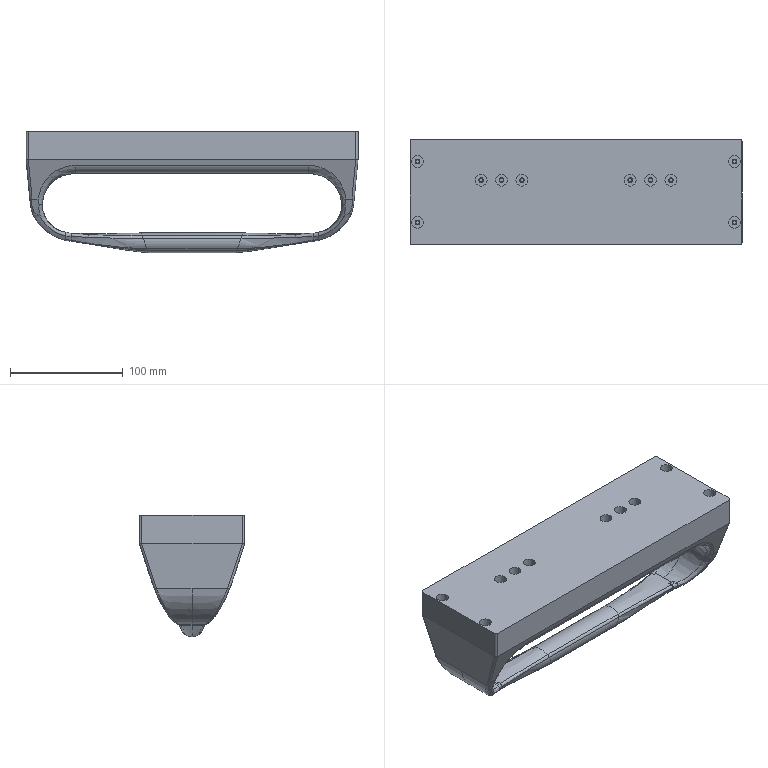NC program | NX | posted with a generic post | part box 294.078 x 93.5 x 107.5 mm
Lines 1 to 258 of 185821:
N10 G17 G21 G94 G90
(ZLEVEL_PROFILE_COPY_COPY_1_COPY_COPY_COPY_COPY_1_COPY , TOOL : D10JING)
N12 T11 M6
N14 G54
N16 G17 G0 G90 X153.539 Y4.496 B0. C0. S7500 M3
N18 G43 Z30. H11
N20 Z-14.083
N22 G94 G1 Z-17.083 F1000.
N24 X153.117 Y4.303
N26 G3 X152.538 Y3.489 R1.
N28 G1 X152.016 Y-1.977
N30 X148.185 Y-41.977
N32 G2 X145.294 Y-52.36 R34.792
N34 X139.783 Y-61.284 R41.542
N36 X129.039 Y-71.069 R47.845
N38 X116.114 Y-77.165 R48.023
N40 X110.357 Y-78.443 R40.705
N42 G1 X107.918 Y-78.805
N44 G3 X84.406 Y-82.6 R3104.615
N46 G2 X61.778 Y-86.214 R2299.005
N48 X52.738 Y-87.55 R870.562
N50 X43.319 Y-88.706 R268.865
N52 X39.042 Y-89. R58.95
N54 G1 X-38.958
N56 G2 X-43.766 Y-88.652 R65.215
N58 X-54.69 Y-87.261 R282.526
N60 X-74.282 Y-84.231 R1365.267
N62 G1 X-80.833 Y-83.169
N64 X-95.124 Y-80.83
N66 X-96.91 Y-80.54
N68 X-107.866 Y-78.799
N70 X-110.27 Y-78.443
N72 G2 X-117.454 Y-76.717 R41.647
N74 X-138.247 Y-63.051 R48.785
N76 X-144.415 Y-54.142 R42.977
N78 X-147.826 Y-44.342 R36.064
N80 X-148.185 Y-41.977 R29.91
N82 G1 X-152.016 Y-1.977
N84 G2 X-152.036 Y-1.675 R5.
N86 G1 X-152.044 Y-1.662
N88 X-152.053 Y-1.578
N90 X-152.539 Y3.496
N92 G3 X-153.119 Y4.31 R1.
N94 G1 X-153.539 Y4.502
N96 Z-14.083
N98 G0 Z30.
N100 X153.539 Y4.495
N102 Z-29.417
N104 G1 Z-32.417
N106 X153.118 Y4.303
N108 G3 X152.538 Y3.489 R1.
N110 G1 X152.016 Y-1.977
N112 X148.185 Y-41.977
N114 G2 X145.589 Y-51.689 R34.666
N116 X140.148 Y-60.823 R41.108
N118 X129.958 Y-70.441 R47.496
N120 X116.114 Y-77.167 R48.183
N122 X110.357 Y-78.443 R40.559
N124 G1 X107.918 Y-78.805
N126 G3 X84.406 Y-82.601 R3047.623
N128 G2 X61.779 Y-86.214 R2288.49
N130 X52.698 Y-87.554 R792.66
N132 X43.319 Y-88.706 R259.673
N134 X39.042 Y-89. R58.502
N136 G1 X-38.958
N138 G2 X-43.766 Y-88.652 R64.859
N140 X-55.824 Y-87.095 R292.145
N142 X-79.047 Y-83.46 R1588.068
N144 G1 X-96.91 Y-80.54
N146 X-107.866 Y-78.799
N148 X-110.27 Y-78.443
N150 G2 X-116.561 Y-77.005 R40.87
N152 X-128.978 Y-71.069 R48.151
N154 X-139.783 Y-61.238 R47.856
N156 X-145.473 Y-51.914 R41.36
N158 X-148.185 Y-41.977 R34.707
N160 G1 X-152.016 Y-1.977
N162 G2 X-152.036 Y-1.675 R5.
N164 G1 X-152.045 Y-1.662
N166 X-152.539 Y3.495
N168 G3 X-153.12 Y4.31 R1.
N170 G1 X-153.54 Y4.501
N172 Z-29.417
N174 G0 Z30.
N176 X153.54 Y4.495
N178 Z-44.75
N180 G1 Z-47.75
N182 X153.119 Y4.303
N184 G3 X152.538 Y3.489 R1.
N186 G1 X152.016 Y-1.977
N188 X148.185 Y-41.977
N190 G2 X145.589 Y-51.69 R34.638
N192 X139.783 Y-61.284 R41.349
N194 X129.512 Y-70.751 R47.668
N196 X117.007 Y-76.892 R48.224
N198 X110.35 Y-78.444 R40.993
N200 G1 X107.918 Y-78.805
N202 G3 X84.406 Y-82.601 R3090.503
N204 G2 X61.779 Y-86.214 R2278.07
N206 X52.698 Y-87.555 R789.646
N208 X43.319 Y-88.707 R261.333
N210 X39.042 Y-89. R58.377
N212 G1 X-38.958
N214 G2 X-43.325 Y-88.698 R61.364
N216 G1 X-44.659 Y-88.557
N218 G2 X-55.824 Y-87.096 R299.771
N220 G1 X-57.164 Y-86.897
N222 G2 X-80.833 Y-83.17 R1733.297
N224 G1 X-96.91 Y-80.541
N226 X-107.866 Y-78.799
N228 X-110.266 Y-78.444
N230 G2 X-115.667 Y-77.272 R39.927
N232 X-128.979 Y-71.069 R48.025
N234 X-139.783 Y-61.238 R47.852
N236 X-145.474 Y-51.914 R41.354
N238 X-148.185 Y-41.977 R34.724
N240 G1 X-152.016 Y-1.977
N242 G2 X-152.036 Y-1.675 R5.
N244 G1 X-152.046 Y-1.662
N246 X-152.54 Y3.495
N248 G3 X-153.121 Y4.31 R1.
N250 G1 X-153.54 Y4.501
N252 Z-44.75
N254 G0 Z30.
(ZLEVEL_PROFILE_COPY_COPY_1_COPY_COPY_COPY_COPY_1 , TOOL : D10JING)
N256 X-112.33 Y-59.814
N258 Z-12.917
N260 G1 Z-15.917
N262 X-112.118 Y-60.353
N264 G3 X-111.336 Y-60.977 R1.
N266 G1 X-106.464 Y-61.713
N268 G3 X-97.301 Y-62.063 R216.41
N270 X-81.073 Y-62.143 R607.517
N272 X-57.618 Y-61.793 R1794.406
N274 G1 X-53.058 Y-61.695
N276 X-45.461 Y-61.511
N278 X-45.014 Y-61.501
N280 X45.258 Y-61.504
N282 G3 X77.434 Y-62.111 R2132.135
N284 X93.969 Y-62.12 R742.157
N286 X102.013 Y-61.933 R361.575
N288 X108.406 Y-61.583 R149.493
N290 G1 X108.716 Y-61.559
N292 G3 X116.314 Y-59.378 R19.201
N294 X125.325 Y-50.638 R22.338
N296 X127.29 Y-45.73 R19.465
N298 X127.767 Y-41.952 R16.012
N300 G1 X127.769 Y-41.703
N302 G3 X123.962 Y-29.194 R22.015
N304 X116.314 Y-22.034 R23.863
N306 X103.263 Y-18.5 R25.703
N308 G1 X-103.167
N310 G3 X-116.235 Y-22.046 R25.697
N312 X-124.561 Y-30.289 R23.699
N314 X-127.673 Y-41.703 R21.924
N316 G1 X-127.671 Y-42.149
N318 G3 X-127.381 Y-44.83 R14.436
N320 X-126.125 Y-48.851 R17.708
N322 X-121.433 Y-55.568 R21.749
N324 X-114.729 Y-60.081 R21.718
N326 X-112.942 Y-60.732 R16.267
N328 G1 X-111.757 Y-60.913
N330 G2 X-111.336 Y-60.977 R1.828
N332 G3 X-110.853 Y-60.85 R0.5
N334 G1 X-110.141 Y-60.146
N336 Z-12.917
N338 G0 Z30.
N340 X-112.151 Y-59.841
N342 Z-28.833
N344 G1 Z-31.833
N346 X-112.04 Y-60.266
N348 G3 X-111.336 Y-60.977 R1.
N350 G1 X-106.464 Y-61.713
N352 G3 X-97.301 Y-62.063 R216.391
N354 X-81.073 Y-62.143 R607.506
N356 X-57.618 Y-61.793 R1794.39
N358 G1 X-53.058 Y-61.695
N360 X-45.461 Y-61.511
N362 X-45.014 Y-61.501
N364 X45.258 Y-61.504
N366 G3 X77.434 Y-62.111 R2132.136
N368 X93.969 Y-62.12 R742.141
N370 X102.013 Y-61.933 R361.594
N372 X108.406 Y-61.583 R149.495
N374 G1 X108.716 Y-61.559
N376 G3 X116.314 Y-59.378 R19.201
N378 X125.325 Y-50.638 R22.338
N380 X127.29 Y-45.731 R19.464
N382 X127.767 Y-41.945 R16.009
N384 G1 X127.769 Y-41.703
N386 G3 X123.961 Y-29.194 R22.015
N388 X116.314 Y-22.035 R23.86
N390 X103.257 Y-18.5 R25.706
N392 G1 X-103.167
N394 G3 X-116.235 Y-22.046 R25.703
N396 X-124.561 Y-30.289 R23.703
N398 X-127.672 Y-41.703 R21.922
N400 G1 X-127.671 Y-42.149
N402 G3 X-127.381 Y-44.83 R14.432
N404 X-126.125 Y-48.851 R17.708
N406 X-121.433 Y-55.568 R21.749
N408 X-114.729 Y-60.081 R21.718
N410 X-112.942 Y-60.732 R16.267
N412 G1 X-111.757 Y-60.913
N414 G2 X-111.336 Y-60.977 R1.828
N416 G3 X-110.853 Y-60.85 R0.5
N418 G1 X-110.141 Y-60.146
N420 Z-28.833
N422 G0 Z30.
N424 X-112.151 Y-59.841
N426 Z-44.75
N428 G1 Z-47.75
N430 X-112.04 Y-60.266
N432 G3 X-111.336 Y-60.977 R1.
N434 G1 X-106.464 Y-61.713
N436 G3 X-97.301 Y-62.063 R216.373
N438 X-81.075 Y-62.143 R607.495
N440 X-57.62 Y-61.793 R1794.03
N442 G1 X-53.058 Y-61.695
N444 X-45.461 Y-61.511
N446 X-45.014 Y-61.501
N448 X45.258 Y-61.504
N450 G3 X77.434 Y-62.111 R2132.136
N452 X93.969 Y-62.12 R742.126
N454 X102.013 Y-61.933 R361.614
N456 X108.406 Y-61.583 R149.497
N458 G1 X108.716 Y-61.559
N460 G3 X116.314 Y-59.378 R19.201
N462 X125.325 Y-50.638 R22.338
N464 X127.29 Y-45.731 R19.464
N466 X127.767 Y-41.945 R16.009
N468 G1 X127.769 Y-41.703
N470 G3 X123.961 Y-29.194 R22.015
N472 X116.314 Y-22.035 R23.86
N474 X103.257 Y-18.5 R25.706
N476 G1 X-103.167
N478 G3 X-116.235 Y-22.046 R25.703
N480 X-124.561 Y-30.289 R23.703
N482 X-127.672 Y-41.703 R21.922
N484 G1 X-127.671 Y-42.149
N486 G3 X-127.381 Y-44.83 R14.432
N488 X-126.125 Y-48.851 R17.708
N490 X-121.433 Y-55.568 R21.749
N492 X-114.729 Y-60.081 R21.719
N494 X-112.942 Y-60.732 R16.267
N496 G1 X-111.757 Y-60.913
N498 G2 X-111.336 Y-60.977 R1.827
N500 G3 X-110.853 Y-60.85 R0.5
N502 G1 X-110.141 Y-60.146
N504 Z-44.75
N506 G0 Z30.
N508 M5